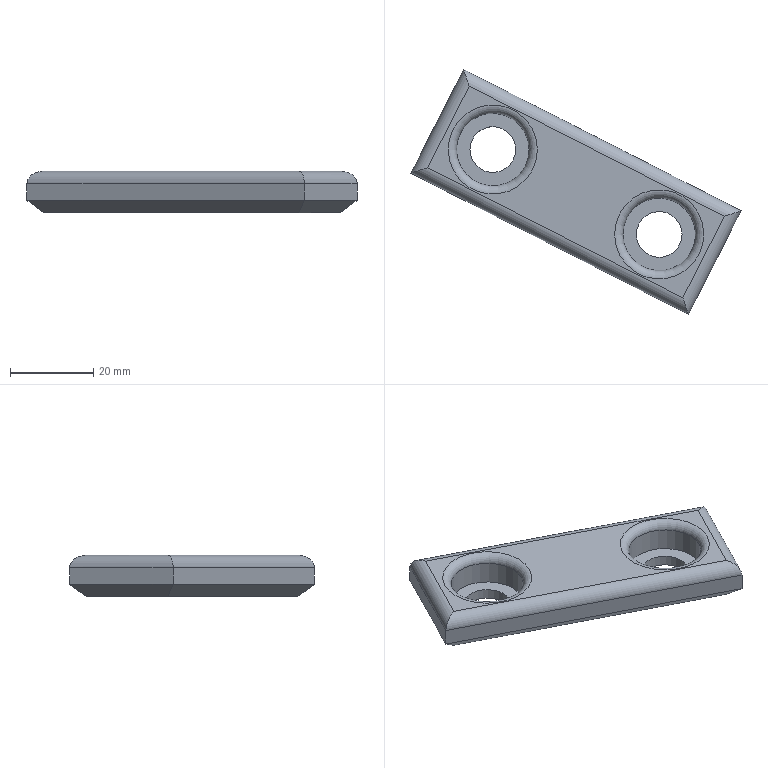Part | STEP file | gslz 2016.10.28-13_id1814_x_t | 1 solid | 145 faces | box 79.537 x 58.997 x 10 mm | volume 15532 mm3 | plane 100 | other 35 | cylinder 8 | torus 2 | commonest cylinder face diameters 6 x4 11 x2 17.5 x2